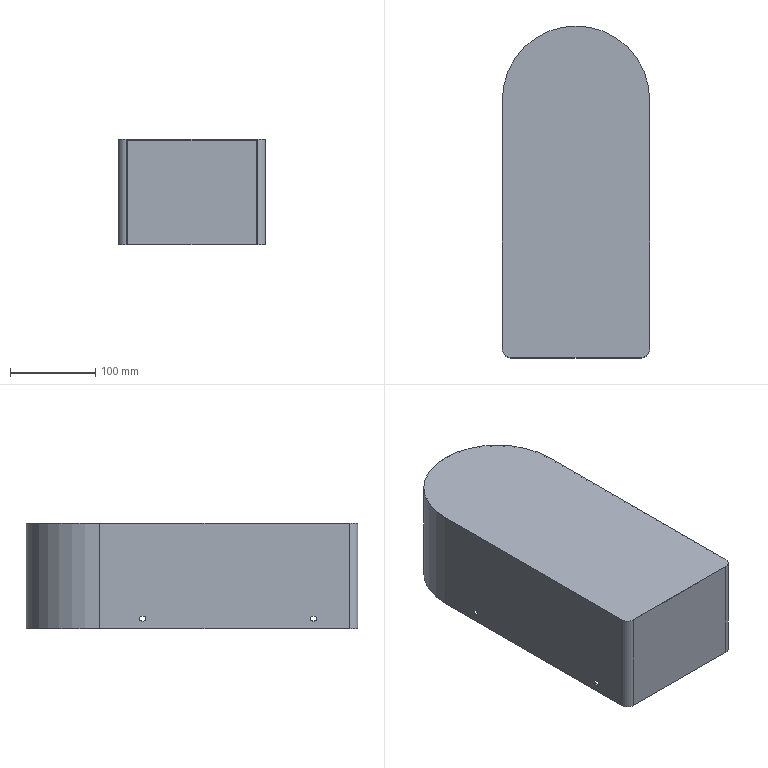Part | SolidWorks | features Fillet 2, ICE 2, Extrusion 1 | 1 solid | 31 faces | box 172.4 x 388.4 x 123 mm | volume 228799 mm3 | plane 17 | cylinder 14 | commonest cylinder face diameters 5.5 x8 20 x4 170 x1 172.4 x1
STEP:
#1=CARTESIAN_POINT('',(85.,150.5,121.8));
#2=VERTEX_POINT('',#1);
#3=CARTESIAN_POINT('',(85.,150.5,0.));
#4=VERTEX_POINT('',#3);
#5=CARTESIAN_POINT('',(85.,150.5,123.));
#6=DIRECTION('',(0.,0.,-1.));
#7=VECTOR('',#6,1000.);
#8=LINE('',#5,#7);
#9=EDGE_CURVE('',#2,#4,#8,.T.);
#10=ORIENTED_EDGE('',*,*,#9,.F.);
#11=CARTESIAN_POINT('',(-85.,150.5,121.8));
#12=VERTEX_POINT('',#11);
#13=CARTESIAN_POINT('',(0.,150.5,121.8));
#14=DIRECTION('',(0.,0.,1.));
#15=DIRECTION('',(1.,0.,0.));
#16=AXIS2_PLACEMENT_3D('',#13,#14,#15);
#17=CIRCLE('',#16,85.);
#18=EDGE_CURVE('',#2,#12,#17,.T.);
#19=ORIENTED_EDGE('',*,*,#18,.T.);
#20=CARTESIAN_POINT('',(-85.,150.5,0.));
#21=VERTEX_POINT('',#20);
#22=CARTESIAN_POINT('',(-85.,150.5,123.));
#23=DIRECTION('',(0.,0.,-1.));
#24=VECTOR('',#23,1000.);
#25=LINE('',#22,#24);
#26=EDGE_CURVE('',#12,#21,#25,.T.);
#27=ORIENTED_EDGE('',*,*,#26,.T.);
#28=CARTESIAN_POINT('',(0.,150.5,0.));
#29=DIRECTION('',(0.,0.,1.));
#30=DIRECTION('',(1.,0.,0.));
#31=AXIS2_PLACEMENT_3D('',#28,#29,#30);
#32=CIRCLE('',#31,85.);
#33=EDGE_CURVE('',#4,#21,#32,.T.);
#34=ORIENTED_EDGE('',*,*,#33,.F.);
#35=EDGE_LOOP('',(#10,#19,#27,#34));
#36=FACE_OUTER_BOUND('',#35,.T.);
#37=CARTESIAN_POINT('',(0.,150.5,123.));
#38=DIRECTION('',(0.,0.,-1.));
#39=DIRECTION('',(-1.,0.,0.));
#40=AXIS2_PLACEMENT_3D('',#37,#38,#39);
#41=CYLINDRICAL_SURFACE('',#40,85.);
#42=ADVANCED_FACE('',(#36),#41,.F.);
#43=CARTESIAN_POINT('',(-85.,99.3,14.25));
#44=VERTEX_POINT('',#43);
#45=CARTESIAN_POINT('',(-85.,99.3,8.75));
#46=VERTEX_POINT('',#45);
#47=CARTESIAN_POINT('',(-85.,99.3,11.5));
#48=DIRECTION('',(1.,0.,0.));
#49=DIRECTION('',(0.,0.,-1.));
#50=AXIS2_PLACEMENT_3D('',#47,#48,#49);
#51=CIRCLE('',#50,2.75);
#52=EDGE_CURVE('',#44,#46,#51,.T.);
#53=ORIENTED_EDGE('',*,*,#52,.F.);
#54=CARTESIAN_POINT('',(-85.,101.3,14.25));
#55=VERTEX_POINT('',#54);
#56=CARTESIAN_POINT('',(-85.,-140.5,14.25));
#57=DIRECTION('',(0.,-1.,0.));
#58=VECTOR('',#57,1000.);
#59=LINE('',#56,#58);
#60=EDGE_CURVE('',#55,#44,#59,.T.);
#61=ORIENTED_EDGE('',*,*,#60,.F.);
#62=CARTESIAN_POINT('',(-85.,101.3,8.75));
#63=VERTEX_POINT('',#62);
#64=CARTESIAN_POINT('',(-85.,101.3,11.5));
#65=DIRECTION('',(1.,0.,0.));
#66=DIRECTION('',(0.,0.,-1.));
#67=AXIS2_PLACEMENT_3D('',#64,#65,#66);
#68=CIRCLE('',#67,2.75);
#69=EDGE_CURVE('',#63,#55,#68,.T.);
#70=ORIENTED_EDGE('',*,*,#69,.F.);
#71=CARTESIAN_POINT('',(-85.,-140.5,8.75));
#72=DIRECTION('',(0.,1.,0.));
#73=VECTOR('',#72,1000.);
#74=LINE('',#71,#73);
#75=EDGE_CURVE('',#46,#63,#74,.T.);
#76=ORIENTED_EDGE('',*,*,#75,.F.);
#77=EDGE_LOOP('',(#53,#61,#70,#76));
#78=FACE_BOUND('',#77,.T.);
#79=CARTESIAN_POINT('',(-85.,-100.7,14.25));
#80=VERTEX_POINT('',#79);
#81=CARTESIAN_POINT('',(-85.,-100.7,8.75));
#82=VERTEX_POINT('',#81);
#83=CARTESIAN_POINT('',(-85.,-100.7,11.5));
#84=DIRECTION('',(1.,0.,0.));
#85=DIRECTION('',(0.,0.,-1.));
#86=AXIS2_PLACEMENT_3D('',#83,#84,#85);
#87=CIRCLE('',#86,2.75);
#88=EDGE_CURVE('',#80,#82,#87,.T.);
#89=ORIENTED_EDGE('',*,*,#88,.F.);
#90=CARTESIAN_POINT('',(-85.,-98.7,14.25));
#91=VERTEX_POINT('',#90);
#92=CARTESIAN_POINT('',(-85.,-140.5,14.25));
#93=DIRECTION('',(0.,-1.,0.));
#94=VECTOR('',#93,1000.);
#95=LINE('',#92,#94);
#96=EDGE_CURVE('',#91,#80,#95,.T.);
#97=ORIENTED_EDGE('',*,*,#96,.F.);
#98=CARTESIAN_POINT('',(-85.,-98.7,8.75));
#99=VERTEX_POINT('',#98);
#100=CARTESIAN_POINT('',(-85.,-98.7,11.5));
#101=DIRECTION('',(1.,0.,0.));
#102=DIRECTION('',(0.,0.,-1.));
#103=AXIS2_PLACEMENT_3D('',#100,#101,#102);
#104=CIRCLE('',#103,2.75);
#105=EDGE_CURVE('',#99,#91,#104,.T.);
#106=ORIENTED_EDGE('',*,*,#105,.F.);
#107=CARTESIAN_POINT('',(-85.,-140.5,8.75));
#108=DIRECTION('',(0.,1.,0.));
#109=VECTOR('',#108,1000.);
#110=LINE('',#107,#109);
#111=EDGE_CURVE('',#82,#99,#110,.T.);
#112=ORIENTED_EDGE('',*,*,#111,.F.);
#113=EDGE_LOOP('',(#89,#97,#106,#112));
#114=FACE_BOUND('',#113,.T.);
#115=ORIENTED_EDGE('',*,*,#26,.F.);
#116=CARTESIAN_POINT('',(-85.,-140.5,121.8));
#117=VERTEX_POINT('',#116);
#118=CARTESIAN_POINT('',(-85.,-140.5,121.8));
#119=DIRECTION('',(0.,-1.,0.));
#120=VECTOR('',#119,1000.);
#121=LINE('',#118,#120);
#122=EDGE_CURVE('',#12,#117,#121,.T.);
#123=ORIENTED_EDGE('',*,*,#122,.T.);
#124=CARTESIAN_POINT('',(-85.,-140.5,0.));
#125=VERTEX_POINT('',#124);
#126=CARTESIAN_POINT('',(-85.,-140.5,123.));
#127=DIRECTION('',(0.,0.,-1.));
#128=VECTOR('',#127,1000.);
#129=LINE('',#126,#128);
#130=EDGE_CURVE('',#117,#125,#129,.T.);
#131=ORIENTED_EDGE('',*,*,#130,.T.);
#132=CARTESIAN_POINT('',(-85.,-140.5,0.));
#133=DIRECTION('',(0.,-1.,0.));
#134=VECTOR('',#133,1000.);
#135=LINE('',#132,#134);
#136=EDGE_CURVE('',#21,#125,#135,.T.);
#137=ORIENTED_EDGE('',*,*,#136,.F.);
#138=EDGE_LOOP('',(#115,#123,#131,#137));
#139=FACE_OUTER_BOUND('',#138,.T.);
#140=CARTESIAN_POINT('',(-85.,-140.5,123.));
#141=DIRECTION('',(1.,0.,0.));
#142=DIRECTION('',(0.,0.,-1.));
#143=AXIS2_PLACEMENT_3D('',#140,#141,#142);
#144=PLANE('',#143);
#145=ADVANCED_FACE('',(#78,#114,#139),#144,.T.);
#146=ORIENTED_EDGE('',*,*,#130,.F.);
#147=CARTESIAN_POINT('',(-75.,-150.5,121.8));
#148=VERTEX_POINT('',#147);
#149=CARTESIAN_POINT('',(-75.,-140.5,121.8));
#150=DIRECTION('',(0.,0.,1.));
#151=DIRECTION('',(1.,0.,0.));
#152=AXIS2_PLACEMENT_3D('',#149,#150,#151);
#153=CIRCLE('',#152,10.);
#154=EDGE_CURVE('',#117,#148,#153,.T.);
#155=ORIENTED_EDGE('',*,*,#154,.T.);
#156=CARTESIAN_POINT('',(-75.,-150.5,0.));
#157=VERTEX_POINT('',#156);
#158=CARTESIAN_POINT('',(-75.,-150.5,123.));
#159=DIRECTION('',(0.,0.,-1.));
#160=VECTOR('',#159,1000.);
#161=LINE('',#158,#160);
#162=EDGE_CURVE('',#148,#157,#161,.T.);
#163=ORIENTED_EDGE('',*,*,#162,.T.);
#164=CARTESIAN_POINT('',(-75.,-140.5,0.));
#165=DIRECTION('',(0.,0.,1.));
#166=DIRECTION('',(1.,0.,0.));
#167=AXIS2_PLACEMENT_3D('',#164,#165,#166);
#168=CIRCLE('',#167,10.);
#169=EDGE_CURVE('',#125,#157,#168,.T.);
#170=ORIENTED_EDGE('',*,*,#169,.F.);
#171=EDGE_LOOP('',(#146,#155,#163,#170));
#172=FACE_OUTER_BOUND('',#171,.T.);
#173=CARTESIAN_POINT('',(-75.,-140.5,123.));
#174=DIRECTION('',(0.,0.,-1.));
#175=DIRECTION('',(-1.,0.,0.));
#176=AXIS2_PLACEMENT_3D('',#173,#174,#175);
#177=CYLINDRICAL_SURFACE('',#176,10.);
#178=ADVANCED_FACE('',(#172),#177,.F.);
#179=ORIENTED_EDGE('',*,*,#162,.F.);
#180=CARTESIAN_POINT('',(75.,-150.5,121.8));
#181=VERTEX_POINT('',#180);
#182=CARTESIAN_POINT('',(75.,-150.5,121.8));
#183=DIRECTION('',(1.,0.,0.));
#184=VECTOR('',#183,1000.);
#185=LINE('',#182,#184);
#186=EDGE_CURVE('',#148,#181,#185,.T.);
#187=ORIENTED_EDGE('',*,*,#186,.T.);
#188=CARTESIAN_POINT('',(75.,-150.5,0.));
#189=VERTEX_POINT('',#188);
#190=CARTESIAN_POINT('',(75.,-150.5,123.));
#191=DIRECTION('',(0.,0.,-1.));
#192=VECTOR('',#191,1000.);
#193=LINE('',#190,#192);
#194=EDGE_CURVE('',#181,#189,#193,.T.);
#195=ORIENTED_EDGE('',*,*,#194,.T.);
#196=CARTESIAN_POINT('',(75.,-150.5,0.));
#197=DIRECTION('',(1.,0.,0.));
#198=VECTOR('',#197,1000.);
#199=LINE('',#196,#198);
#200=EDGE_CURVE('',#157,#189,#199,.T.);
#201=ORIENTED_EDGE('',*,*,#200,.F.);
#202=EDGE_LOOP('',(#179,#187,#195,#201));
#203=FACE_OUTER_BOUND('',#202,.T.);
#204=CARTESIAN_POINT('',(75.,-150.5,123.));
#205=DIRECTION('',(0.,1.,0.));
#206=DIRECTION('',(-1.,0.,0.));
#207=AXIS2_PLACEMENT_3D('',#204,#205,#206);
#208=PLANE('',#207);
#209=ADVANCED_FACE('',(#203),#208,.T.);
#210=ORIENTED_EDGE('',*,*,#194,.F.);
#211=CARTESIAN_POINT('',(85.,-140.5,121.8));
#212=VERTEX_POINT('',#211);
#213=CARTESIAN_POINT('',(75.,-140.5,121.8));
#214=DIRECTION('',(0.,0.,1.));
#215=DIRECTION('',(1.,0.,0.));
#216=AXIS2_PLACEMENT_3D('',#213,#214,#215);
#217=CIRCLE('',#216,10.);
#218=EDGE_CURVE('',#181,#212,#217,.T.);
#219=ORIENTED_EDGE('',*,*,#218,.T.);
#220=CARTESIAN_POINT('',(85.,-140.5,0.));
#221=VERTEX_POINT('',#220);
#222=CARTESIAN_POINT('',(85.,-140.5,123.));
#223=DIRECTION('',(0.,0.,-1.));
#224=VECTOR('',#223,1000.);
#225=LINE('',#222,#224);
#226=EDGE_CURVE('',#212,#221,#225,.T.);
#227=ORIENTED_EDGE('',*,*,#226,.T.);
#228=CARTESIAN_POINT('',(75.,-140.5,0.));
#229=DIRECTION('',(0.,0.,1.));
#230=DIRECTION('',(1.,0.,0.));
#231=AXIS2_PLACEMENT_3D('',#228,#229,#230);
#232=CIRCLE('',#231,10.);
#233=EDGE_CURVE('',#189,#221,#232,.T.);
#234=ORIENTED_EDGE('',*,*,#233,.F.);
#235=EDGE_LOOP('',(#210,#219,#227,#234));
#236=FACE_OUTER_BOUND('',#235,.T.);
#237=CARTESIAN_POINT('',(75.,-140.5,123.));
#238=DIRECTION('',(0.,0.,-1.));
#239=DIRECTION('',(-1.,0.,0.));
#240=AXIS2_PLACEMENT_3D('',#237,#238,#239);
#241=CYLINDRICAL_SURFACE('',#240,10.);
#242=ADVANCED_FACE('',(#236),#241,.F.);
#243=CARTESIAN_POINT('',(85.,99.3,8.75));
#244=VERTEX_POINT('',#243);
#245=CARTESIAN_POINT('',(85.,99.3,14.25));
#246=VERTEX_POINT('',#245);
#247=CARTESIAN_POINT('',(85.,99.3,11.5));
#248=DIRECTION('',(-1.,0.,0.));
#249=DIRECTION('',(0.,0.,1.));
#250=AXIS2_PLACEMENT_3D('',#247,#248,#249);
#251=CIRCLE('',#250,2.75);
#252=EDGE_CURVE('',#244,#246,#251,.T.);
#253=ORIENTED_EDGE('',*,*,#252,.F.);
#254=CARTESIAN_POINT('',(85.,101.3,8.75));
#255=VERTEX_POINT('',#254);
#256=CARTESIAN_POINT('',(85.,-140.5,8.75));
#257=DIRECTION('',(0.,-1.,0.));
#258=VECTOR('',#257,1000.);
#259=LINE('',#256,#258);
#260=EDGE_CURVE('',#255,#244,#259,.T.);
#261=ORIENTED_EDGE('',*,*,#260,.F.);
#262=CARTESIAN_POINT('',(85.,101.3,14.25));
#263=VERTEX_POINT('',#262);
#264=CARTESIAN_POINT('',(85.,101.3,11.5));
#265=DIRECTION('',(-1.,0.,0.));
#266=DIRECTION('',(0.,0.,1.));
#267=AXIS2_PLACEMENT_3D('',#264,#265,#266);
#268=CIRCLE('',#267,2.75);
#269=EDGE_CURVE('',#263,#255,#268,.T.);
#270=ORIENTED_EDGE('',*,*,#269,.F.);
#271=CARTESIAN_POINT('',(85.,-140.5,14.25));
#272=DIRECTION('',(0.,1.,0.));
#273=VECTOR('',#272,1000.);
#274=LINE('',#271,#273);
#275=EDGE_CURVE('',#246,#263,#274,.T.);
#276=ORIENTED_EDGE('',*,*,#275,.F.);
#277=EDGE_LOOP('',(#253,#261,#270,#276));
#278=FACE_BOUND('',#277,.T.);
#279=CARTESIAN_POINT('',(85.,-100.7,8.75));
#280=VERTEX_POINT('',#279);
#281=CARTESIAN_POINT('',(85.,-100.7,14.25));
#282=VERTEX_POINT('',#281);
#283=CARTESIAN_POINT('',(85.,-100.7,11.5));
#284=DIRECTION('',(-1.,0.,0.));
#285=DIRECTION('',(0.,0.,1.));
#286=AXIS2_PLACEMENT_3D('',#283,#284,#285);
#287=CIRCLE('',#286,2.75);
#288=EDGE_CURVE('',#280,#282,#287,.T.);
#289=ORIENTED_EDGE('',*,*,#288,.F.);
#290=CARTESIAN_POINT('',(85.,-98.7,8.75));
#291=VERTEX_POINT('',#290);
#292=CARTESIAN_POINT('',(85.,-140.5,8.75));
#293=DIRECTION('',(0.,-1.,0.));
#294=VECTOR('',#293,1000.);
#295=LINE('',#292,#294);
#296=EDGE_CURVE('',#291,#280,#295,.T.);
#297=ORIENTED_EDGE('',*,*,#296,.F.);
#298=CARTESIAN_POINT('',(85.,-98.7,14.25));
#299=VERTEX_POINT('',#298);
#300=CARTESIAN_POINT('',(85.,-98.7,11.5));
#301=DIRECTION('',(-1.,0.,0.));
#302=DIRECTION('',(0.,0.,1.));
#303=AXIS2_PLACEMENT_3D('',#300,#301,#302);
#304=CIRCLE('',#303,2.75);
#305=EDGE_CURVE('',#299,#291,#304,.T.);
#306=ORIENTED_EDGE('',*,*,#305,.F.);
#307=CARTESIAN_POINT('',(85.,-140.5,14.25));
#308=DIRECTION('',(0.,1.,0.));
#309=VECTOR('',#308,1000.);
#310=LINE('',#307,#309);
#311=EDGE_CURVE('',#282,#299,#310,.T.);
#312=ORIENTED_EDGE('',*,*,#311,.F.);
#313=EDGE_LOOP('',(#289,#297,#306,#312));
#314=FACE_BOUND('',#313,.T.);
#315=ORIENTED_EDGE('',*,*,#226,.F.);
#316=CARTESIAN_POINT('',(85.,-140.5,121.8));
#317=DIRECTION('',(0.,1.,0.));
#318=VECTOR('',#317,1000.);
#319=LINE('',#316,#318);
#320=EDGE_CURVE('',#212,#2,#319,.T.);
#321=ORIENTED_EDGE('',*,*,#320,.T.);
#322=ORIENTED_EDGE('',*,*,#9,.T.);
#323=CARTESIAN_POINT('',(85.,-140.5,0.));
#324=DIRECTION('',(0.,1.,0.));
#325=VECTOR('',#324,1000.);
#326=LINE('',#323,#325);
#327=EDGE_CURVE('',#221,#4,#326,.T.);
#328=ORIENTED_EDGE('',*,*,#327,.F.);
#329=EDGE_LOOP('',(#315,#321,#322,#328));
#330=FACE_OUTER_BOUND('',#329,.T.);
#331=CARTESIAN_POINT('',(85.,-140.5,123.));
#332=DIRECTION('',(-1.,0.,0.));
#333=DIRECTION('',(0.,0.,1.));
#334=AXIS2_PLACEMENT_3D('',#331,#332,#333);
#335=PLANE('',#334);
#336=ADVANCED_FACE('',(#278,#314,#330),#335,.T.);
#337=CARTESIAN_POINT('',(-76.2,-151.7,123.));
#338=VERTEX_POINT('',#337);
#339=CARTESIAN_POINT('',(76.2,-151.7,123.));
#340=VERTEX_POINT('',#339);
#341=CARTESIAN_POINT('',(86.2,-151.7,123.));
#342=DIRECTION('',(1.,0.,0.));
#343=VECTOR('',#342,1000.);
#344=LINE('',#341,#343);
#345=EDGE_CURVE('',#338,#340,#344,.T.);
#346=ORIENTED_EDGE('',*,*,#345,.T.);
#347=CARTESIAN_POINT('',(86.2,-141.7,123.));
#348=VERTEX_POINT('',#347);
#349=CARTESIAN_POINT('',(76.2,-141.7,123.));
#350=DIRECTION('',(0.,0.,1.));
#351=DIRECTION('',(1.,0.,0.));
#352=AXIS2_PLACEMENT_3D('',#349,#350,#351);
#353=CIRCLE('',#352,10.);
#354=EDGE_CURVE('',#340,#348,#353,.T.);
#355=ORIENTED_EDGE('',*,*,#354,.T.);
#356=CARTESIAN_POINT('',(86.2,150.5,123.));
#357=VERTEX_POINT('',#356);
#358=CARTESIAN_POINT('',(86.2,-151.7,123.));
#359=DIRECTION('',(0.,1.,0.));
#360=VECTOR('',#359,1000.);
#361=LINE('',#358,#360);
#362=EDGE_CURVE('',#348,#357,#361,.T.);
#363=ORIENTED_EDGE('',*,*,#362,.T.);
#364=CARTESIAN_POINT('',(-86.2,150.5,123.));
#365=VERTEX_POINT('',#364);
#366=CARTESIAN_POINT('',(0.,150.5,123.));
#367=DIRECTION('',(0.,0.,1.));
#368=DIRECTION('',(1.,0.,0.));
#369=AXIS2_PLACEMENT_3D('',#366,#367,#368);
#370=CIRCLE('',#369,86.2);
#371=EDGE_CURVE('',#357,#365,#370,.T.);
#372=ORIENTED_EDGE('',*,*,#371,.T.);
#373=CARTESIAN_POINT('',(-86.2,-141.7,123.));
#374=VERTEX_POINT('',#373);
#375=CARTESIAN_POINT('',(-86.2,-151.7,123.));
#376=DIRECTION('',(0.,-1.,0.));
#377=VECTOR('',#376,1000.);
#378=LINE('',#375,#377);
#379=EDGE_CURVE('',#365,#374,#378,.T.);
#380=ORIENTED_EDGE('',*,*,#379,.T.);
#381=CARTESIAN_POINT('',(-76.2,-141.7,123.));
#382=DIRECTION('',(0.,0.,1.));
#383=DIRECTION('',(1.,0.,0.));
#384=AXIS2_PLACEMENT_3D('',#381,#382,#383);
#385=CIRCLE('',#384,10.);
#386=EDGE_CURVE('',#374,#338,#385,.T.);
#387=ORIENTED_EDGE('',*,*,#386,.T.);
#388=EDGE_LOOP('',(#346,#355,#363,#372,#380,#387));
#389=FACE_OUTER_BOUND('',#388,.T.);
#390=CARTESIAN_POINT('',(0.,150.5,123.));
#391=DIRECTION('',(0.,0.,1.));
#392=DIRECTION('',(1.,0.,0.));
#393=AXIS2_PLACEMENT_3D('',#390,#391,#392);
#394=PLANE('',#393);
#395=ADVANCED_FACE('',(#389),#394,.T.);
#396=CARTESIAN_POINT('',(86.2,-141.7,0.));
#397=VERTEX_POINT('',#396);
#398=CARTESIAN_POINT('',(86.2,150.5,0.));
#399=VERTEX_POINT('',#398);
#400=CARTESIAN_POINT('',(86.2,-151.7,0.));
#401=DIRECTION('',(0.,1.,0.));
#402=VECTOR('',#401,1000.);
#403=LINE('',#400,#402);
#404=EDGE_CURVE('',#397,#399,#403,.T.);
#405=ORIENTED_EDGE('',*,*,#404,.F.);
#406=CARTESIAN_POINT('',(76.2,-151.7,0.));
#407=VERTEX_POINT('',#406);
#408=CARTESIAN_POINT('',(76.2,-141.7,0.));
#409=DIRECTION('',(0.,0.,-1.));
#410=DIRECTION('',(1.,0.,0.));
#411=AXIS2_PLACEMENT_3D('',#408,#409,#410);
#412=CIRCLE('',#411,10.);
#413=EDGE_CURVE('',#397,#407,#412,.T.);
#414=ORIENTED_EDGE('',*,*,#413,.T.);
#415=CARTESIAN_POINT('',(-76.2,-151.7,0.));
#416=VERTEX_POINT('',#415);
#417=CARTESIAN_POINT('',(86.2,-151.7,0.));
#418=DIRECTION('',(1.,0.,0.));
#419=VECTOR('',#418,1000.);
#420=LINE('',#417,#419);
#421=EDGE_CURVE('',#416,#407,#420,.T.);
#422=ORIENTED_EDGE('',*,*,#421,.F.);
#423=CARTESIAN_POINT('',(-86.2,-141.7,0.));
#424=VERTEX_POINT('',#423);
#425=CARTESIAN_POINT('',(-76.2,-141.7,0.));
#426=DIRECTION('',(0.,0.,-1.));
#427=DIRECTION('',(1.,0.,0.));
#428=AXIS2_PLACEMENT_3D('',#425,#426,#427);
#429=CIRCLE('',#428,10.);
#430=EDGE_CURVE('',#416,#424,#429,.T.);
#431=ORIENTED_EDGE('',*,*,#430,.T.);
#432=CARTESIAN_POINT('',(-86.2,150.5,0.));
#433=VERTEX_POINT('',#432);
#434=CARTESIAN_POINT('',(-86.2,-151.7,0.));
#435=DIRECTION('',(0.,-1.,0.));
#436=VECTOR('',#435,1000.);
#437=LINE('',#434,#436);
#438=EDGE_CURVE('',#433,#424,#437,.T.);
#439=ORIENTED_EDGE('',*,*,#438,.F.);
#440=CARTESIAN_POINT('',(0.,150.5,0.));
#441=DIRECTION('',(0.,0.,1.));
#442=DIRECTION('',(1.,0.,0.));
#443=AXIS2_PLACEMENT_3D('',#440,#441,#442);
#444=CIRCLE('',#443,86.2);
#445=EDGE_CURVE('',#399,#433,#444,.T.);
#446=ORIENTED_EDGE('',*,*,#445,.F.);
#447=EDGE_LOOP('',(#405,#414,#422,#431,#439,#446));
#448=FACE_OUTER_BOUND('',#447,.T.);
#449=ORIENTED_EDGE('',*,*,#33,.T.);
#450=ORIENTED_EDGE('',*,*,#136,.T.);
#451=ORIENTED_EDGE('',*,*,#169,.T.);
#452=ORIENTED_EDGE('',*,*,#200,.T.);
#453=ORIENTED_EDGE('',*,*,#233,.T.);
#454=ORIENTED_EDGE('',*,*,#327,.T.);
#455=EDGE_LOOP('',(#449,#450,#451,#452,#453,#454));
#456=FACE_BOUND('',#455,.T.);
#457=CARTESIAN_POINT('',(0.,150.5,0.));
#458=DIRECTION('',(0.,0.,1.));
#459=DIRECTION('',(1.,0.,0.));
#460=AXIS2_PLACEMENT_3D('',#457,#458,#459);
#461=PLANE('',#460);
#462=ADVANCED_FACE('',(#448,#456),#461,.F.);
#463=CARTESIAN_POINT('',(86.2,150.5,123.));
#464=DIRECTION('',(0.,0.,-1.));
#465=VECTOR('',#464,1000.);
#466=LINE('',#463,#465);
#467=EDGE_CURVE('',#357,#399,#466,.T.);
#468=ORIENTED_EDGE('',*,*,#467,.T.);
#469=ORIENTED_EDGE('',*,*,#445,.T.);
#470=CARTESIAN_POINT('',(-86.2,150.5,123.));
#471=DIRECTION('',(0.,0.,-1.));
#472=VECTOR('',#471,1000.);
#473=LINE('',#470,#472);
#474=EDGE_CURVE('',#365,#433,#473,.T.);
#475=ORIENTED_EDGE('',*,*,#474,.F.);
#476=ORIENTED_EDGE('',*,*,#371,.F.);
#477=EDGE_LOOP('',(#468,#469,#475,#476));
#478=FACE_OUTER_BOUND('',#477,.T.);
#479=CARTESIAN_POINT('',(0.,150.5,123.));
#480=DIRECTION('',(0.,0.,-1.));
#481=DIRECTION('',(-1.,0.,0.));
#482=AXIS2_PLACEMENT_3D('',#479,#480,#481);
#483=CYLINDRICAL_SURFACE('',#482,86.2);
#484=ADVANCED_FACE('',(#478),#483,.T.);
#485=CARTESIAN_POINT('',(-86.2,99.3,14.25));
#486=VERTEX_POINT('',#485);
#487=CARTESIAN_POINT('',(-86.2,101.3,14.25));
#488=VERTEX_POINT('',#487);
#489=CARTESIAN_POINT('',(-86.2,99.3,14.25));
#490=DIRECTION('',(0.,1.,0.));
#491=VECTOR('',#490,1000.);
#492=LINE('',#489,#491);
#493=EDGE_CURVE('',#486,#488,#492,.T.);
#494=ORIENTED_EDGE('',*,*,#493,.F.);
#495=CARTESIAN_POINT('',(-86.2,99.3,8.75));
#496=VERTEX_POINT('',#495);
#497=CARTESIAN_POINT('',(-86.2,99.3,11.5));
#498=DIRECTION('',(-1.,0.,0.));
#499=DIRECTION('',(0.,0.,1.));
#500=AXIS2_PLACEMENT_3D('',#497,#498,#499);
#501=CIRCLE('',#500,2.75);
#502=EDGE_CURVE('',#496,#486,#501,.T.);
#503=ORIENTED_EDGE('',*,*,#502,.F.);
#504=CARTESIAN_POINT('',(-86.2,101.3,8.75));
#505=VERTEX_POINT('',#504);
#506=CARTESIAN_POINT('',(-86.2,99.3,8.75));
#507=DIRECTION('',(0.,-1.,0.));
#508=VECTOR('',#507,1000.);
#509=LINE('',#506,#508);
#510=EDGE_CURVE('',#505,#496,#509,.T.);
#511=ORIENTED_EDGE('',*,*,#510,.F.);
#512=CARTESIAN_POINT('',(-86.2,101.3,11.5));
#513=DIRECTION('',(-1.,0.,0.));
#514=DIRECTION('',(0.,0.,1.));
#515=AXIS2_PLACEMENT_3D('',#512,#513,#514);
#516=CIRCLE('',#515,2.75);
#517=EDGE_CURVE('',#488,#505,#516,.T.);
#518=ORIENTED_EDGE('',*,*,#517,.F.);
#519=EDGE_LOOP('',(#494,#503,#511,#518));
#520=FACE_BOUND('',#519,.T.);
#521=CARTESIAN_POINT('',(-86.2,-100.7,14.25));
#522=VERTEX_POINT('',#521);
#523=CARTESIAN_POINT('',(-86.2,-98.7,14.25));
#524=VERTEX_POINT('',#523);
#525=CARTESIAN_POINT('',(-86.2,-100.7,14.25));
#526=DIRECTION('',(0.,1.,0.));
#527=VECTOR('',#526,1000.);
#528=LINE('',#525,#527);
#529=EDGE_CURVE('',#522,#524,#528,.T.);
#530=ORIENTED_EDGE('',*,*,#529,.F.);
#531=CARTESIAN_POINT('',(-86.2,-100.7,8.75));
#532=VERTEX_POINT('',#531);
#533=CARTESIAN_POINT('',(-86.2,-100.7,11.5));
#534=DIRECTION('',(-1.,0.,0.));
#535=DIRECTION('',(0.,0.,1.));
#536=AXIS2_PLACEMENT_3D('',#533,#534,#535);
#537=CIRCLE('',#536,2.75);
#538=EDGE_CURVE('',#532,#522,#537,.T.);
#539=ORIENTED_EDGE('',*,*,#538,.F.);
#540=CARTESIAN_POINT('',(-86.2,-98.7,8.75));
#541=VERTEX_POINT('',#540);
#542=CARTESIAN_POINT('',(-86.2,-100.7,8.75));
#543=DIRECTION('',(0.,-1.,0.));
#544=VECTOR('',#543,1000.);
#545=LINE('',#542,#544);
#546=EDGE_CURVE('',#541,#532,#545,.T.);
#547=ORIENTED_EDGE('',*,*,#546,.F.);
#548=CARTESIAN_POINT('',(-86.2,-98.7,11.5));
#549=DIRECTION('',(-1.,0.,0.));
#550=DIRECTION('',(0.,0.,1.));
#551=AXIS2_PLACEMENT_3D('',#548,#549,#550);
#552=CIRCLE('',#551,2.75);
#553=EDGE_CURVE('',#524,#541,#552,.T.);
#554=ORIENTED_EDGE('',*,*,#553,.F.);
#555=EDGE_LOOP('',(#530,#539,#547,#554));
#556=FACE_BOUND('',#555,.T.);
#557=ORIENTED_EDGE('',*,*,#438,.T.);
#558=CARTESIAN_POINT('',(-86.2,-141.7,123.));
#559=DIRECTION('',(0.,0.,1.));
#560=VECTOR('',#559,1000.);
#561=LINE('',#558,#560);
#562=EDGE_CURVE('',#424,#374,#561,.T.);
#563=ORIENTED_EDGE('',*,*,#562,.T.);
#564=ORIENTED_EDGE('',*,*,#379,.F.);
#565=ORIENTED_EDGE('',*,*,#474,.T.);
#566=EDGE_LOOP('',(#557,#563,#564,#565));
#567=FACE_OUTER_BOUND('',#566,.T.);
#568=CARTESIAN_POINT('',(-86.2,-151.7,123.));
#569=DIRECTION('',(1.,0.,0.));
#570=DIRECTION('',(0.,0.,-1.));
#571=AXIS2_PLACEMENT_3D('',#568,#569,#570);
#572=PLANE('',#571);
#573=ADVANCED_FACE('',(#520,#556,#567),#572,.F.);
#574=ORIENTED_EDGE('',*,*,#421,.T.);
#575=CARTESIAN_POINT('',(76.2,-151.7,123.));
#576=DIRECTION('',(0.,0.,1.));
#577=VECTOR('',#576,1000.);
#578=LINE('',#575,#577);
#579=EDGE_CURVE('',#407,#340,#578,.T.);
#580=ORIENTED_EDGE('',*,*,#579,.T.);
#581=ORIENTED_EDGE('',*,*,#345,.F.);
#582=CARTESIAN_POINT('',(-76.2,-151.7,123.));
#583=DIRECTION('',(0.,0.,-1.));
#584=VECTOR('',#583,1000.);
#585=LINE('',#582,#584);
#586=EDGE_CURVE('',#338,#416,#585,.T.);
#587=ORIENTED_EDGE('',*,*,#586,.T.);
#588=EDGE_LOOP('',(#574,#580,#581,#587));
#589=FACE_OUTER_BOUND('',#588,.T.);
#590=CARTESIAN_POINT('',(86.2,-151.7,123.));
#591=DIRECTION('',(0.,1.,0.));
#592=DIRECTION('',(-1.,0.,0.));
#593=AXIS2_PLACEMENT_3D('',#590,#591,#592);
#594=PLANE('',#593);
#595=ADVANCED_FACE('',(#589),#594,.F.);
#596=CARTESIAN_POINT('',(86.2,101.3,8.75));
#597=VERTEX_POINT('',#596);
#598=CARTESIAN_POINT('',(86.2,99.3,8.75));
#599=VERTEX_POINT('',#598);
#600=CARTESIAN_POINT('',(86.2,99.3,8.75));
#601=DIRECTION('',(0.,-1.,0.));
#602=VECTOR('',#601,1000.);
#603=LINE('',#600,#602);
#604=EDGE_CURVE('',#597,#599,#603,.T.);
#605=ORIENTED_EDGE('',*,*,#604,.T.);
#606=CARTESIAN_POINT('',(86.2,99.3,14.25));
#607=VERTEX_POINT('',#606);
#608=CARTESIAN_POINT('',(86.2,99.3,11.5));
#609=DIRECTION('',(-1.,0.,0.));
#610=DIRECTION('',(0.,0.,1.));
#611=AXIS2_PLACEMENT_3D('',#608,#609,#610);
#612=CIRCLE('',#611,2.75);
#613=EDGE_CURVE('',#599,#607,#612,.T.);
#614=ORIENTED_EDGE('',*,*,#613,.T.);
#615=CARTESIAN_POINT('',(86.2,101.3,14.25));
#616=VERTEX_POINT('',#615);
#617=CARTESIAN_POINT('',(86.2,99.3,14.25));
#618=DIRECTION('',(0.,1.,0.));
#619=VECTOR('',#618,1000.);
#620=LINE('',#617,#619);
#621=EDGE_CURVE('',#607,#616,#620,.T.);
#622=ORIENTED_EDGE('',*,*,#621,.T.);
#623=CARTESIAN_POINT('',(86.2,101.3,11.5));
#624=DIRECTION('',(-1.,0.,0.));
#625=DIRECTION('',(0.,0.,1.));
#626=AXIS2_PLACEMENT_3D('',#623,#624,#625);
#627=CIRCLE('',#626,2.75);
#628=EDGE_CURVE('',#616,#597,#627,.T.);
#629=ORIENTED_EDGE('',*,*,#628,.T.);
#630=EDGE_LOOP('',(#605,#614,#622,#629));
#631=FACE_BOUND('',#630,.T.);
#632=CARTESIAN_POINT('',(86.2,-98.7,8.75));
#633=VERTEX_POINT('',#632);
#634=CARTESIAN_POINT('',(86.2,-100.7,8.75));
#635=VERTEX_POINT('',#634);
#636=CARTESIAN_POINT('',(86.2,-100.7,8.75));
#637=DIRECTION('',(0.,-1.,0.));
#638=VECTOR('',#637,1000.);
#639=LINE('',#636,#638);
#640=EDGE_CURVE('',#633,#635,#639,.T.);
#641=ORIENTED_EDGE('',*,*,#640,.T.);
#642=CARTESIAN_POINT('',(86.2,-100.7,14.25));
#643=VERTEX_POINT('',#642);
#644=CARTESIAN_POINT('',(86.2,-100.7,11.5));
#645=DIRECTION('',(-1.,0.,0.));
#646=DIRECTION('',(0.,0.,1.));
#647=AXIS2_PLACEMENT_3D('',#644,#645,#646);
#648=CIRCLE('',#647,2.75);
#649=EDGE_CURVE('',#635,#643,#648,.T.);
#650=ORIENTED_EDGE('',*,*,#649,.T.);
#651=CARTESIAN_POINT('',(86.2,-98.7,14.25));
#652=VERTEX_POINT('',#651);
#653=CARTESIAN_POINT('',(86.2,-100.7,14.25));
#654=DIRECTION('',(0.,1.,0.));
#655=VECTOR('',#654,1000.);
#656=LINE('',#653,#655);
#657=EDGE_CURVE('',#643,#652,#656,.T.);
#658=ORIENTED_EDGE('',*,*,#657,.T.);
#659=CARTESIAN_POINT('',(86.2,-98.7,11.5));
#660=DIRECTION('',(-1.,0.,0.));
#661=DIRECTION('',(0.,0.,1.));
#662=AXIS2_PLACEMENT_3D('',#659,#660,#661);
#663=CIRCLE('',#662,2.75);
#664=EDGE_CURVE('',#652,#633,#663,.T.);
#665=ORIENTED_EDGE('',*,*,#664,.T.);
#666=EDGE_LOOP('',(#641,#650,#658,#665));
#667=FACE_BOUND('',#666,.T.);
#668=ORIENTED_EDGE('',*,*,#362,.F.);
#669=CARTESIAN_POINT('',(86.2,-141.7,123.));
#670=DIRECTION('',(0.,0.,-1.));
#671=VECTOR('',#670,1000.);
#672=LINE('',#669,#671);
#673=EDGE_CURVE('',#348,#397,#672,.T.);
#674=ORIENTED_EDGE('',*,*,#673,.T.);
#675=ORIENTED_EDGE('',*,*,#404,.T.);
#676=ORIENTED_EDGE('',*,*,#467,.F.);
#677=EDGE_LOOP('',(#668,#674,#675,#676));
#678=FACE_OUTER_BOUND('',#677,.T.);
#679=CARTESIAN_POINT('',(86.2,-151.7,123.));
#680=DIRECTION('',(-1.,0.,0.));
#681=DIRECTION('',(0.,0.,1.));
#682=AXIS2_PLACEMENT_3D('',#679,#680,#681);
#683=PLANE('',#682);
#684=ADVANCED_FACE('',(#631,#667,#678),#683,.F.);
#685=ORIENTED_EDGE('',*,*,#18,.F.);
#686=ORIENTED_EDGE('',*,*,#320,.F.);
#687=ORIENTED_EDGE('',*,*,#218,.F.);
#688=ORIENTED_EDGE('',*,*,#186,.F.);
#689=ORIENTED_EDGE('',*,*,#154,.F.);
#690=ORIENTED_EDGE('',*,*,#122,.F.);
#691=EDGE_LOOP('',(#685,#686,#687,#688,#689,#690));
#692=FACE_OUTER_BOUND('',#691,.T.);
#693=CARTESIAN_POINT('',(0.,150.5,121.8));
#694=DIRECTION('',(0.,0.,1.));
#695=DIRECTION('',(1.,0.,0.));
#696=AXIS2_PLACEMENT_3D('',#693,#694,#695);
#697=PLANE('',#696);
#698=ADVANCED_FACE('',(#692),#697,.F.);
#699=ORIENTED_EDGE('',*,*,#386,.F.);
#700=ORIENTED_EDGE('',*,*,#562,.F.);
#701=ORIENTED_EDGE('',*,*,#430,.F.);
#702=ORIENTED_EDGE('',*,*,#586,.F.);
#703=EDGE_LOOP('',(#699,#700,#701,#702));
#704=FACE_OUTER_BOUND('',#703,.T.);
#705=CARTESIAN_POINT('',(-76.2,-141.7,123.));
#706=DIRECTION('',(0.,0.,-1.));
#707=DIRECTION('',(-1.,0.,0.));
#708=AXIS2_PLACEMENT_3D('',#705,#706,#707);
#709=CYLINDRICAL_SURFACE('',#708,10.);
#710=ADVANCED_FACE('',(#704),#709,.T.);
#711=ORIENTED_EDGE('',*,*,#354,.F.);
#712=ORIENTED_EDGE('',*,*,#579,.F.);
#713=ORIENTED_EDGE('',*,*,#413,.F.);
#714=ORIENTED_EDGE('',*,*,#673,.F.);
#715=EDGE_LOOP('',(#711,#712,#713,#714));
#716=FACE_OUTER_BOUND('',#715,.T.);
#717=CARTESIAN_POINT('',(76.2,-141.7,123.));
#718=DIRECTION('',(0.,0.,-1.));
#719=DIRECTION('',(-1.,0.,0.));
#720=AXIS2_PLACEMENT_3D('',#717,#718,#719);
#721=CYLINDRICAL_SURFACE('',#720,10.);
#722=ADVANCED_FACE('',(#716),#721,.T.);
#723=ORIENTED_EDGE('',*,*,#311,.T.);
#724=CARTESIAN_POINT('',(86.2,-98.7,14.25));
#725=DIRECTION('',(-1.,0.,0.));
#726=VECTOR('',#725,1000.);
#727=LINE('',#724,#726);
#728=EDGE_CURVE('',#652,#299,#727,.T.);
#729=ORIENTED_EDGE('',*,*,#728,.F.);
#730=ORIENTED_EDGE('',*,*,#657,.F.);
#731=CARTESIAN_POINT('',(86.2,-100.7,14.25));
#732=DIRECTION('',(-1.,0.,0.));
#733=VECTOR('',#732,1000.);
#734=LINE('',#731,#733);
#735=EDGE_CURVE('',#643,#282,#734,.T.);
#736=ORIENTED_EDGE('',*,*,#735,.T.);
#737=EDGE_LOOP('',(#723,#729,#730,#736));
#738=FACE_OUTER_BOUND('',#737,.T.);
#739=CARTESIAN_POINT('',(86.2,-100.7,14.25));
#740=DIRECTION('',(0.,0.,1.));
#741=DIRECTION('',(1.,0.,0.));
#742=AXIS2_PLACEMENT_3D('',#739,#740,#741);
#743=PLANE('',#742);
#744=ADVANCED_FACE('',(#738),#743,.F.);
#745=ORIENTED_EDGE('',*,*,#305,.T.);
#746=CARTESIAN_POINT('',(86.2,-98.7,8.75));
#747=DIRECTION('',(-1.,0.,0.));
#748=VECTOR('',#747,1000.);
#749=LINE('',#746,#748);
#750=EDGE_CURVE('',#633,#291,#749,.T.);
#751=ORIENTED_EDGE('',*,*,#750,.F.);
#752=ORIENTED_EDGE('',*,*,#664,.F.);
#753=ORIENTED_EDGE('',*,*,#728,.T.);
#754=EDGE_LOOP('',(#745,#751,#752,#753));
#755=FACE_OUTER_BOUND('',#754,.T.);
#756=CARTESIAN_POINT('',(86.2,-98.7,11.5));
#757=DIRECTION('',(-1.,0.,0.));
#758=DIRECTION('',(0.,0.,1.));
#759=AXIS2_PLACEMENT_3D('',#756,#757,#758);
#760=CYLINDRICAL_SURFACE('',#759,2.75);
#761=ADVANCED_FACE('',(#755),#760,.F.);
#762=ORIENTED_EDGE('',*,*,#296,.T.);
#763=CARTESIAN_POINT('',(86.2,-100.7,8.75));
#764=DIRECTION('',(-1.,0.,0.));
#765=VECTOR('',#764,1000.);
#766=LINE('',#763,#765);
#767=EDGE_CURVE('',#635,#280,#766,.T.);
#768=ORIENTED_EDGE('',*,*,#767,.F.);
#769=ORIENTED_EDGE('',*,*,#640,.F.);
#770=ORIENTED_EDGE('',*,*,#750,.T.);
#771=EDGE_LOOP('',(#762,#768,#769,#770));
#772=FACE_OUTER_BOUND('',#771,.T.);
#773=CARTESIAN_POINT('',(86.2,-100.7,8.75));
#774=DIRECTION('',(0.,0.,-1.));
#775=DIRECTION('',(-1.,0.,0.));
#776=AXIS2_PLACEMENT_3D('',#773,#774,#775);
#777=PLANE('',#776);
#778=ADVANCED_FACE('',(#772),#777,.F.);
#779=ORIENTED_EDGE('',*,*,#288,.T.);
#780=ORIENTED_EDGE('',*,*,#735,.F.);
#781=ORIENTED_EDGE('',*,*,#649,.F.);
#782=ORIENTED_EDGE('',*,*,#767,.T.);
#783=EDGE_LOOP('',(#779,#780,#781,#782));
#784=FACE_OUTER_BOUND('',#783,.T.);
#785=CARTESIAN_POINT('',(86.2,-100.7,11.5));
#786=DIRECTION('',(-1.,0.,0.));
#787=DIRECTION('',(0.,0.,1.));
#788=AXIS2_PLACEMENT_3D('',#785,#786,#787);
#789=CYLINDRICAL_SURFACE('',#788,2.75);
#790=ADVANCED_FACE('',(#784),#789,.F.);
#791=ORIENTED_EDGE('',*,*,#275,.T.);
#792=CARTESIAN_POINT('',(86.2,101.3,14.25));
#793=DIRECTION('',(-1.,0.,0.));
#794=VECTOR('',#793,1000.);
#795=LINE('',#792,#794);
#796=EDGE_CURVE('',#616,#263,#795,.T.);
#797=ORIENTED_EDGE('',*,*,#796,.F.);
#798=ORIENTED_EDGE('',*,*,#621,.F.);
#799=CARTESIAN_POINT('',(86.2,99.3,14.25));
#800=DIRECTION('',(-1.,0.,0.));
#801=VECTOR('',#800,1000.);
#802=LINE('',#799,#801);
#803=EDGE_CURVE('',#607,#246,#802,.T.);
#804=ORIENTED_EDGE('',*,*,#803,.T.);
#805=EDGE_LOOP('',(#791,#797,#798,#804));
#806=FACE_OUTER_BOUND('',#805,.T.);
#807=CARTESIAN_POINT('',(86.2,99.3,14.25));
#808=DIRECTION('',(0.,0.,1.));
#809=DIRECTION('',(1.,0.,0.));
#810=AXIS2_PLACEMENT_3D('',#807,#808,#809);
#811=PLANE('',#810);
#812=ADVANCED_FACE('',(#806),#811,.F.);
#813=ORIENTED_EDGE('',*,*,#269,.T.);
#814=CARTESIAN_POINT('',(86.2,101.3,8.75));
#815=DIRECTION('',(-1.,0.,0.));
#816=VECTOR('',#815,1000.);
#817=LINE('',#814,#816);
#818=EDGE_CURVE('',#597,#255,#817,.T.);
#819=ORIENTED_EDGE('',*,*,#818,.F.);
#820=ORIENTED_EDGE('',*,*,#628,.F.);
#821=ORIENTED_EDGE('',*,*,#796,.T.);
#822=EDGE_LOOP('',(#813,#819,#820,#821));
#823=FACE_OUTER_BOUND('',#822,.T.);
#824=CARTESIAN_POINT('',(86.2,101.3,11.5));
#825=DIRECTION('',(-1.,0.,0.));
#826=DIRECTION('',(0.,0.,1.));
#827=AXIS2_PLACEMENT_3D('',#824,#825,#826);
#828=CYLINDRICAL_SURFACE('',#827,2.75);
#829=ADVANCED_FACE('',(#823),#828,.F.);
#830=ORIENTED_EDGE('',*,*,#260,.T.);
#831=CARTESIAN_POINT('',(86.2,99.3,8.75));
#832=DIRECTION('',(-1.,0.,0.));
#833=VECTOR('',#832,1000.);
#834=LINE('',#831,#833);
#835=EDGE_CURVE('',#599,#244,#834,.T.);
#836=ORIENTED_EDGE('',*,*,#835,.F.);
#837=ORIENTED_EDGE('',*,*,#604,.F.);
#838=ORIENTED_EDGE('',*,*,#818,.T.);
#839=EDGE_LOOP('',(#830,#836,#837,#838));
#840=FACE_OUTER_BOUND('',#839,.T.);
#841=CARTESIAN_POINT('',(86.2,99.3,8.75));
#842=DIRECTION('',(0.,0.,-1.));
#843=DIRECTION('',(-1.,0.,0.));
#844=AXIS2_PLACEMENT_3D('',#841,#842,#843);
#845=PLANE('',#844);
#846=ADVANCED_FACE('',(#840),#845,.F.);
#847=ORIENTED_EDGE('',*,*,#252,.T.);
#848=ORIENTED_EDGE('',*,*,#803,.F.);
#849=ORIENTED_EDGE('',*,*,#613,.F.);
#850=ORIENTED_EDGE('',*,*,#835,.T.);
#851=EDGE_LOOP('',(#847,#848,#849,#850));
#852=FACE_OUTER_BOUND('',#851,.T.);
#853=CARTESIAN_POINT('',(86.2,99.3,11.5));
#854=DIRECTION('',(-1.,0.,0.));
#855=DIRECTION('',(0.,0.,1.));
#856=AXIS2_PLACEMENT_3D('',#853,#854,#855);
#857=CYLINDRICAL_SURFACE('',#856,2.75);
#858=ADVANCED_FACE('',(#852),#857,.F.);
#859=ORIENTED_EDGE('',*,*,#88,.T.);
#860=CARTESIAN_POINT('',(86.2,-100.7,8.75));
#861=DIRECTION('',(-1.,0.,0.));
#862=VECTOR('',#861,1000.);
#863=LINE('',#860,#862);
#864=EDGE_CURVE('',#82,#532,#863,.T.);
#865=ORIENTED_EDGE('',*,*,#864,.T.);
#866=ORIENTED_EDGE('',*,*,#538,.T.);
#867=CARTESIAN_POINT('',(86.2,-100.7,14.25));
#868=DIRECTION('',(-1.,0.,0.));
#869=VECTOR('',#868,1000.);
#870=LINE('',#867,#869);
#871=EDGE_CURVE('',#80,#522,#870,.T.);
#872=ORIENTED_EDGE('',*,*,#871,.F.);
#873=EDGE_LOOP('',(#859,#865,#866,#872));
#874=FACE_OUTER_BOUND('',#873,.T.);
#875=CARTESIAN_POINT('',(86.2,-100.7,11.5));
#876=DIRECTION('',(-1.,0.,0.));
#877=DIRECTION('',(0.,0.,1.));
#878=AXIS2_PLACEMENT_3D('',#875,#876,#877);
#879=CYLINDRICAL_SURFACE('',#878,2.75);
#880=ADVANCED_FACE('',(#874),#879,.F.);
#881=ORIENTED_EDGE('',*,*,#111,.T.);
#882=CARTESIAN_POINT('',(86.2,-98.7,8.75));
#883=DIRECTION('',(-1.,0.,0.));
#884=VECTOR('',#883,1000.);
#885=LINE('',#882,#884);
#886=EDGE_CURVE('',#99,#541,#885,.T.);
#887=ORIENTED_EDGE('',*,*,#886,.T.);
#888=ORIENTED_EDGE('',*,*,#546,.T.);
#889=ORIENTED_EDGE('',*,*,#864,.F.);
#890=EDGE_LOOP('',(#881,#887,#888,#889));
#891=FACE_OUTER_BOUND('',#890,.T.);
#892=CARTESIAN_POINT('',(86.2,-100.7,8.75));
#893=DIRECTION('',(0.,0.,-1.));
#894=DIRECTION('',(-1.,0.,0.));
#895=AXIS2_PLACEMENT_3D('',#892,#893,#894);
#896=PLANE('',#895);
#897=ADVANCED_FACE('',(#891),#896,.F.);
#898=ORIENTED_EDGE('',*,*,#105,.T.);
#899=CARTESIAN_POINT('',(86.2,-98.7,14.25));
#900=DIRECTION('',(-1.,0.,0.));
#901=VECTOR('',#900,1000.);
#902=LINE('',#899,#901);
#903=EDGE_CURVE('',#91,#524,#902,.T.);
#904=ORIENTED_EDGE('',*,*,#903,.T.);
#905=ORIENTED_EDGE('',*,*,#553,.T.);
#906=ORIENTED_EDGE('',*,*,#886,.F.);
#907=EDGE_LOOP('',(#898,#904,#905,#906));
#908=FACE_OUTER_BOUND('',#907,.T.);
#909=CARTESIAN_POINT('',(86.2,-98.7,11.5));
#910=DIRECTION('',(-1.,0.,0.));
#911=DIRECTION('',(0.,0.,1.));
#912=AXIS2_PLACEMENT_3D('',#909,#910,#911);
#913=CYLINDRICAL_SURFACE('',#912,2.75);
#914=ADVANCED_FACE('',(#908),#913,.F.);
#915=ORIENTED_EDGE('',*,*,#96,.T.);
#916=ORIENTED_EDGE('',*,*,#871,.T.);
#917=ORIENTED_EDGE('',*,*,#529,.T.);
#918=ORIENTED_EDGE('',*,*,#903,.F.);
#919=EDGE_LOOP('',(#915,#916,#917,#918));
#920=FACE_OUTER_BOUND('',#919,.T.);
#921=CARTESIAN_POINT('',(86.2,-100.7,14.25));
#922=DIRECTION('',(0.,0.,1.));
#923=DIRECTION('',(1.,0.,0.));
#924=AXIS2_PLACEMENT_3D('',#921,#922,#923);
#925=PLANE('',#924);
#926=ADVANCED_FACE('',(#920),#925,.F.);
#927=ORIENTED_EDGE('',*,*,#52,.T.);
#928=CARTESIAN_POINT('',(86.2,99.3,8.75));
#929=DIRECTION('',(-1.,0.,0.));
#930=VECTOR('',#929,1000.);
#931=LINE('',#928,#930);
#932=EDGE_CURVE('',#46,#496,#931,.T.);
#933=ORIENTED_EDGE('',*,*,#932,.T.);
#934=ORIENTED_EDGE('',*,*,#502,.T.);
#935=CARTESIAN_POINT('',(86.2,99.3,14.25));
#936=DIRECTION('',(-1.,0.,0.));
#937=VECTOR('',#936,1000.);
#938=LINE('',#935,#937);
#939=EDGE_CURVE('',#44,#486,#938,.T.);
#940=ORIENTED_EDGE('',*,*,#939,.F.);
#941=EDGE_LOOP('',(#927,#933,#934,#940));
#942=FACE_OUTER_BOUND('',#941,.T.);
#943=CARTESIAN_POINT('',(86.2,99.3,11.5));
#944=DIRECTION('',(-1.,0.,0.));
#945=DIRECTION('',(0.,0.,1.));
#946=AXIS2_PLACEMENT_3D('',#943,#944,#945);
#947=CYLINDRICAL_SURFACE('',#946,2.75);
#948=ADVANCED_FACE('',(#942),#947,.F.);
#949=ORIENTED_EDGE('',*,*,#75,.T.);
#950=CARTESIAN_POINT('',(86.2,101.3,8.75));
#951=DIRECTION('',(-1.,0.,0.));
#952=VECTOR('',#951,1000.);
#953=LINE('',#950,#952);
#954=EDGE_CURVE('',#63,#505,#953,.T.);
#955=ORIENTED_EDGE('',*,*,#954,.T.);
#956=ORIENTED_EDGE('',*,*,#510,.T.);
#957=ORIENTED_EDGE('',*,*,#932,.F.);
#958=EDGE_LOOP('',(#949,#955,#956,#957));
#959=FACE_OUTER_BOUND('',#958,.T.);
#960=CARTESIAN_POINT('',(86.2,99.3,8.75));
#961=DIRECTION('',(0.,0.,-1.));
#962=DIRECTION('',(-1.,0.,0.));
#963=AXIS2_PLACEMENT_3D('',#960,#961,#962);
#964=PLANE('',#963);
#965=ADVANCED_FACE('',(#959),#964,.F.);
#966=ORIENTED_EDGE('',*,*,#69,.T.);
#967=CARTESIAN_POINT('',(86.2,101.3,14.25));
#968=DIRECTION('',(-1.,0.,0.));
#969=VECTOR('',#968,1000.);
#970=LINE('',#967,#969);
#971=EDGE_CURVE('',#55,#488,#970,.T.);
#972=ORIENTED_EDGE('',*,*,#971,.T.);
#973=ORIENTED_EDGE('',*,*,#517,.T.);
#974=ORIENTED_EDGE('',*,*,#954,.F.);
#975=EDGE_LOOP('',(#966,#972,#973,#974));
#976=FACE_OUTER_BOUND('',#975,.T.);
#977=CARTESIAN_POINT('',(86.2,101.3,11.5));
#978=DIRECTION('',(-1.,0.,0.));
#979=DIRECTION('',(0.,0.,1.));
#980=AXIS2_PLACEMENT_3D('',#977,#978,#979);
#981=CYLINDRICAL_SURFACE('',#980,2.75);
#982=ADVANCED_FACE('',(#976),#981,.F.);
#983=ORIENTED_EDGE('',*,*,#60,.T.);
#984=ORIENTED_EDGE('',*,*,#939,.T.);
#985=ORIENTED_EDGE('',*,*,#493,.T.);
#986=ORIENTED_EDGE('',*,*,#971,.F.);
#987=EDGE_LOOP('',(#983,#984,#985,#986));
#988=FACE_OUTER_BOUND('',#987,.T.);
#989=CARTESIAN_POINT('',(86.2,99.3,14.25));
#990=DIRECTION('',(0.,0.,1.));
#991=DIRECTION('',(1.,0.,0.));
#992=AXIS2_PLACEMENT_3D('',#989,#990,#991);
#993=PLANE('',#992);
#994=ADVANCED_FACE('',(#988),#993,.F.);
#995=CLOSED_SHELL('',(#42,#145,#178,#209,#242,#336,#395,#462,#484,#573,#595,#684,#698,#710,#722,#744,#761,#778,#790,#812,#829,#846,#858,#880,#897,#914,#926,#948,#965,#982,#994));
#996=MANIFOLD_SOLID_BREP('',#995);
#997=CARTESIAN_POINT('',(0.,0.,0.));
#998=DIRECTION('',(0.,0.,1.));
#999=DIRECTION('',(1.,0.,0.));
#1000=AXIS2_PLACEMENT_3D('',#997,#998,#999);
#1001=(LENGTH_UNIT()NAMED_UNIT(*)SI_UNIT(.MILLI.,.METRE.));
#1002=UNCERTAINTY_MEASURE_WITH_UNIT(LENGTH_MEASURE(0.00001),#1001,'','');
#1003=(NAMED_UNIT(*)PLANE_ANGLE_UNIT()SI_UNIT($,.RADIAN.));
#1004=(NAMED_UNIT(*)SI_UNIT($,.STERADIAN.)SOLID_ANGLE_UNIT());
#1005=(GEOMETRIC_REPRESENTATION_CONTEXT(3)GLOBAL_UNCERTAINTY_ASSIGNED_CONTEXT((#1002))GLOBAL_UNIT_ASSIGNED_CONTEXT((#1001,#1003,#1004))REPRESENTATION_CONTEXT('',''));
#1006=ADVANCED_BREP_SHAPE_REPRESENTATION('',(#996,#1000),#1005);